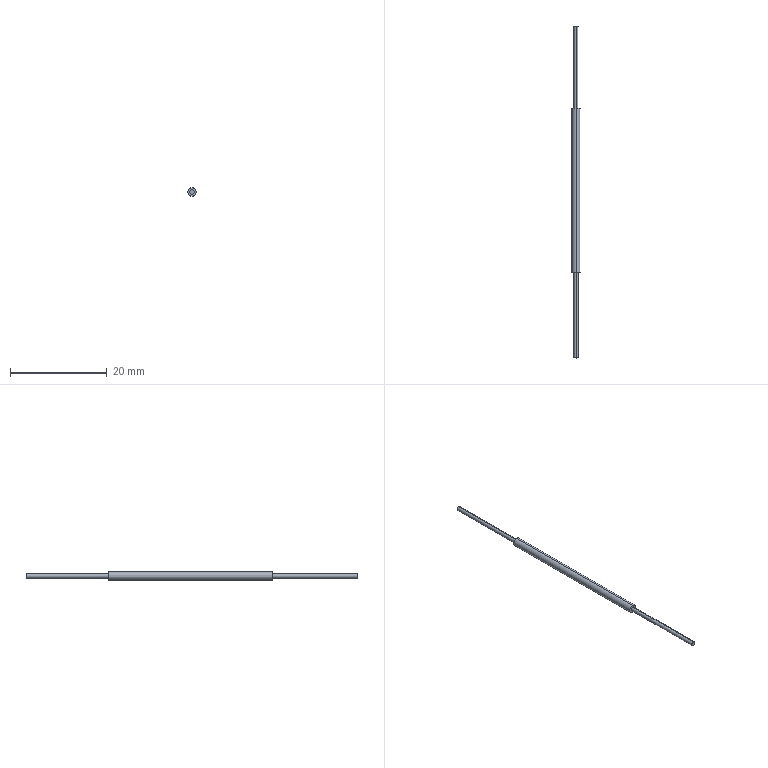Part | SolidWorks | features Revolution 1 | 1 solid | 10 faces | box 1.75 x 68.75 x 1.75 mm | volume 103.887 mm3 | cylinder 6 | plane 4 | commonest cylinder face diameters 0.9 x4 1.75 x2
STEP:
#1=CARTESIAN_POINT('',(0.,67.,-0.45));
#2=VERTEX_POINT('',#1);
#3=CARTESIAN_POINT('',(0.,67.,0.45));
#4=VERTEX_POINT('',#3);
#5=CARTESIAN_POINT('',(0.,67.,0.));
#6=DIRECTION('',(0.,-1.,0.));
#7=DIRECTION('',(0.,0.,-1.));
#8=AXIS2_PLACEMENT_3D('',#5,#6,#7);
#9=CIRCLE('',#8,0.45);
#10=EDGE_CURVE('',#2,#4,#9,.T.);
#11=ORIENTED_EDGE('',*,*,#10,.T.);
#12=CARTESIAN_POINT('',(0.,50.,0.45));
#13=VERTEX_POINT('',#12);
#14=CARTESIAN_POINT('',(0.,-4.379,0.45));
#15=DIRECTION('',(0.,-1.,0.));
#16=VECTOR('',#15,1000.);
#17=LINE('',#14,#16);
#18=EDGE_CURVE('',#4,#13,#17,.T.);
#19=ORIENTED_EDGE('',*,*,#18,.T.);
#20=CARTESIAN_POINT('',(0.,50.,-0.45));
#21=VERTEX_POINT('',#20);
#22=CARTESIAN_POINT('',(0.,50.,0.));
#23=DIRECTION('',(0.,-1.,0.));
#24=DIRECTION('',(0.,0.,-1.));
#25=AXIS2_PLACEMENT_3D('',#22,#23,#24);
#26=CIRCLE('',#25,0.45);
#27=EDGE_CURVE('',#21,#13,#26,.T.);
#28=ORIENTED_EDGE('',*,*,#27,.F.);
#29=CARTESIAN_POINT('',(0.,-4.379,-0.45));
#30=DIRECTION('',(0.,-1.,0.));
#31=VECTOR('',#30,1000.);
#32=LINE('',#29,#31);
#33=EDGE_CURVE('',#2,#21,#32,.T.);
#34=ORIENTED_EDGE('',*,*,#33,.F.);
#35=EDGE_LOOP('',(#11,#19,#28,#34));
#36=FACE_OUTER_BOUND('',#35,.T.);
#37=CARTESIAN_POINT('',(0.,-4.379,0.));
#38=DIRECTION('',(0.,-1.,0.));
#39=DIRECTION('',(0.,0.,-1.));
#40=AXIS2_PLACEMENT_3D('',#37,#38,#39);
#41=CYLINDRICAL_SURFACE('',#40,0.45);
#42=ADVANCED_FACE('',(#36),#41,.T.);
#43=CARTESIAN_POINT('',(0.,50.,-0.875));
#44=VERTEX_POINT('',#43);
#45=CARTESIAN_POINT('',(0.,50.,0.875));
#46=VERTEX_POINT('',#45);
#47=CARTESIAN_POINT('',(0.,50.,0.));
#48=DIRECTION('',(0.,-1.,0.));
#49=DIRECTION('',(0.,0.,-1.));
#50=AXIS2_PLACEMENT_3D('',#47,#48,#49);
#51=CIRCLE('',#50,0.875);
#52=EDGE_CURVE('',#44,#46,#51,.T.);
#53=ORIENTED_EDGE('',*,*,#52,.T.);
#54=CARTESIAN_POINT('',(0.,16.,0.875));
#55=VERTEX_POINT('',#54);
#56=CARTESIAN_POINT('',(0.,-4.379,0.875));
#57=DIRECTION('',(0.,-1.,0.));
#58=VECTOR('',#57,1000.);
#59=LINE('',#56,#58);
#60=EDGE_CURVE('',#46,#55,#59,.T.);
#61=ORIENTED_EDGE('',*,*,#60,.T.);
#62=CARTESIAN_POINT('',(0.,16.,-0.875));
#63=VERTEX_POINT('',#62);
#64=CARTESIAN_POINT('',(0.,16.,0.));
#65=DIRECTION('',(0.,-1.,0.));
#66=DIRECTION('',(0.,0.,-1.));
#67=AXIS2_PLACEMENT_3D('',#64,#65,#66);
#68=CIRCLE('',#67,0.875);
#69=EDGE_CURVE('',#63,#55,#68,.T.);
#70=ORIENTED_EDGE('',*,*,#69,.F.);
#71=CARTESIAN_POINT('',(0.,-4.379,-0.875));
#72=DIRECTION('',(0.,-1.,0.));
#73=VECTOR('',#72,1000.);
#74=LINE('',#71,#73);
#75=EDGE_CURVE('',#44,#63,#74,.T.);
#76=ORIENTED_EDGE('',*,*,#75,.F.);
#77=EDGE_LOOP('',(#53,#61,#70,#76));
#78=FACE_OUTER_BOUND('',#77,.T.);
#79=CARTESIAN_POINT('',(0.,-4.379,0.));
#80=DIRECTION('',(0.,-1.,0.));
#81=DIRECTION('',(0.,0.,-1.));
#82=AXIS2_PLACEMENT_3D('',#79,#80,#81);
#83=CYLINDRICAL_SURFACE('',#82,0.875);
#84=ADVANCED_FACE('',(#78),#83,.T.);
#85=CARTESIAN_POINT('',(0.,16.,-0.45));
#86=VERTEX_POINT('',#85);
#87=CARTESIAN_POINT('',(0.,16.,0.45));
#88=VERTEX_POINT('',#87);
#89=CARTESIAN_POINT('',(0.,16.,0.));
#90=DIRECTION('',(0.,-1.,0.));
#91=DIRECTION('',(0.,0.,-1.));
#92=AXIS2_PLACEMENT_3D('',#89,#90,#91);
#93=CIRCLE('',#92,0.45);
#94=EDGE_CURVE('',#86,#88,#93,.T.);
#95=ORIENTED_EDGE('',*,*,#94,.T.);
#96=CARTESIAN_POINT('',(0.,-1.75,0.45));
#97=VERTEX_POINT('',#96);
#98=CARTESIAN_POINT('',(0.,-4.379,0.45));
#99=DIRECTION('',(0.,-1.,0.));
#100=VECTOR('',#99,1000.);
#101=LINE('',#98,#100);
#102=EDGE_CURVE('',#88,#97,#101,.T.);
#103=ORIENTED_EDGE('',*,*,#102,.T.);
#104=CARTESIAN_POINT('',(0.,-1.75,-0.45));
#105=VERTEX_POINT('',#104);
#106=CARTESIAN_POINT('',(0.,-1.75,0.));
#107=DIRECTION('',(0.,-1.,0.));
#108=DIRECTION('',(0.,0.,-1.));
#109=AXIS2_PLACEMENT_3D('',#106,#107,#108);
#110=CIRCLE('',#109,0.45);
#111=EDGE_CURVE('',#105,#97,#110,.T.);
#112=ORIENTED_EDGE('',*,*,#111,.F.);
#113=CARTESIAN_POINT('',(0.,-4.379,-0.45));
#114=DIRECTION('',(0.,-1.,0.));
#115=VECTOR('',#114,1000.);
#116=LINE('',#113,#115);
#117=EDGE_CURVE('',#86,#105,#116,.T.);
#118=ORIENTED_EDGE('',*,*,#117,.F.);
#119=EDGE_LOOP('',(#95,#103,#112,#118));
#120=FACE_OUTER_BOUND('',#119,.T.);
#121=CARTESIAN_POINT('',(0.,-4.379,0.));
#122=DIRECTION('',(0.,-1.,0.));
#123=DIRECTION('',(0.,0.,-1.));
#124=AXIS2_PLACEMENT_3D('',#121,#122,#123);
#125=CYLINDRICAL_SURFACE('',#124,0.45);
#126=ADVANCED_FACE('',(#120),#125,.T.);
#127=ORIENTED_EDGE('',*,*,#10,.F.);
#128=CARTESIAN_POINT('',(0.,67.,0.));
#129=DIRECTION('',(0.,-1.,0.));
#130=DIRECTION('',(0.,0.,-1.));
#131=AXIS2_PLACEMENT_3D('',#128,#129,#130);
#132=CIRCLE('',#131,0.45);
#133=EDGE_CURVE('',#4,#2,#132,.T.);
#134=ORIENTED_EDGE('',*,*,#133,.F.);
#135=EDGE_LOOP('',(#127,#134));
#136=FACE_OUTER_BOUND('',#135,.T.);
#137=CARTESIAN_POINT('',(0.,67.,-0.45));
#138=DIRECTION('',(0.,1.,0.));
#139=DIRECTION('',(0.,0.,1.));
#140=AXIS2_PLACEMENT_3D('',#137,#138,#139);
#141=PLANE('',#140);
#142=ADVANCED_FACE('',(#136),#141,.T.);
#143=ORIENTED_EDGE('',*,*,#111,.T.);
#144=CARTESIAN_POINT('',(0.,-1.75,0.));
#145=DIRECTION('',(0.,-1.,0.));
#146=DIRECTION('',(0.,0.,-1.));
#147=AXIS2_PLACEMENT_3D('',#144,#145,#146);
#148=CIRCLE('',#147,0.45);
#149=EDGE_CURVE('',#97,#105,#148,.T.);
#150=ORIENTED_EDGE('',*,*,#149,.T.);
#151=EDGE_LOOP('',(#143,#150));
#152=FACE_OUTER_BOUND('',#151,.T.);
#153=CARTESIAN_POINT('',(0.,-1.75,0.));
#154=DIRECTION('',(0.,-1.,0.));
#155=DIRECTION('',(0.,0.,-1.));
#156=AXIS2_PLACEMENT_3D('',#153,#154,#155);
#157=PLANE('',#156);
#158=ADVANCED_FACE('',(#152),#157,.T.);
#159=ORIENTED_EDGE('',*,*,#102,.F.);
#160=CARTESIAN_POINT('',(0.,16.,0.));
#161=DIRECTION('',(0.,-1.,0.));
#162=DIRECTION('',(0.,0.,-1.));
#163=AXIS2_PLACEMENT_3D('',#160,#161,#162);
#164=CIRCLE('',#163,0.45);
#165=EDGE_CURVE('',#88,#86,#164,.T.);
#166=ORIENTED_EDGE('',*,*,#165,.T.);
#167=ORIENTED_EDGE('',*,*,#117,.T.);
#168=ORIENTED_EDGE('',*,*,#149,.F.);
#169=EDGE_LOOP('',(#159,#166,#167,#168));
#170=FACE_OUTER_BOUND('',#169,.T.);
#171=CARTESIAN_POINT('',(0.,-4.379,0.));
#172=DIRECTION('',(0.,-1.,0.));
#173=DIRECTION('',(0.,0.,-1.));
#174=AXIS2_PLACEMENT_3D('',#171,#172,#173);
#175=CYLINDRICAL_SURFACE('',#174,0.45);
#176=ADVANCED_FACE('',(#170),#175,.T.);
#177=ORIENTED_EDGE('',*,*,#69,.T.);
#178=CARTESIAN_POINT('',(0.,16.,0.));
#179=DIRECTION('',(0.,-1.,0.));
#180=DIRECTION('',(0.,0.,-1.));
#181=AXIS2_PLACEMENT_3D('',#178,#179,#180);
#182=CIRCLE('',#181,0.875);
#183=EDGE_CURVE('',#55,#63,#182,.T.);
#184=ORIENTED_EDGE('',*,*,#183,.T.);
#185=EDGE_LOOP('',(#177,#184));
#186=FACE_OUTER_BOUND('',#185,.T.);
#187=ORIENTED_EDGE('',*,*,#94,.F.);
#188=ORIENTED_EDGE('',*,*,#165,.F.);
#189=EDGE_LOOP('',(#187,#188));
#190=FACE_BOUND('',#189,.T.);
#191=CARTESIAN_POINT('',(0.,16.,-0.45));
#192=DIRECTION('',(0.,-1.,0.));
#193=DIRECTION('',(0.,0.,-1.));
#194=AXIS2_PLACEMENT_3D('',#191,#192,#193);
#195=PLANE('',#194);
#196=ADVANCED_FACE('',(#186,#190),#195,.T.);
#197=ORIENTED_EDGE('',*,*,#60,.F.);
#198=CARTESIAN_POINT('',(0.,50.,0.));
#199=DIRECTION('',(0.,-1.,0.));
#200=DIRECTION('',(0.,0.,-1.));
#201=AXIS2_PLACEMENT_3D('',#198,#199,#200);
#202=CIRCLE('',#201,0.875);
#203=EDGE_CURVE('',#46,#44,#202,.T.);
#204=ORIENTED_EDGE('',*,*,#203,.T.);
#205=ORIENTED_EDGE('',*,*,#75,.T.);
#206=ORIENTED_EDGE('',*,*,#183,.F.);
#207=EDGE_LOOP('',(#197,#204,#205,#206));
#208=FACE_OUTER_BOUND('',#207,.T.);
#209=CARTESIAN_POINT('',(0.,-4.379,0.));
#210=DIRECTION('',(0.,-1.,0.));
#211=DIRECTION('',(0.,0.,-1.));
#212=AXIS2_PLACEMENT_3D('',#209,#210,#211);
#213=CYLINDRICAL_SURFACE('',#212,0.875);
#214=ADVANCED_FACE('',(#208),#213,.T.);
#215=ORIENTED_EDGE('',*,*,#27,.T.);
#216=CARTESIAN_POINT('',(0.,50.,0.));
#217=DIRECTION('',(0.,-1.,0.));
#218=DIRECTION('',(0.,0.,-1.));
#219=AXIS2_PLACEMENT_3D('',#216,#217,#218);
#220=CIRCLE('',#219,0.45);
#221=EDGE_CURVE('',#13,#21,#220,.T.);
#222=ORIENTED_EDGE('',*,*,#221,.T.);
#223=EDGE_LOOP('',(#215,#222));
#224=FACE_BOUND('',#223,.T.);
#225=ORIENTED_EDGE('',*,*,#52,.F.);
#226=ORIENTED_EDGE('',*,*,#203,.F.);
#227=EDGE_LOOP('',(#225,#226));
#228=FACE_OUTER_BOUND('',#227,.T.);
#229=CARTESIAN_POINT('',(0.,50.,-0.875));
#230=DIRECTION('',(0.,1.,0.));
#231=DIRECTION('',(0.,0.,1.));
#232=AXIS2_PLACEMENT_3D('',#229,#230,#231);
#233=PLANE('',#232);
#234=ADVANCED_FACE('',(#224,#228),#233,.T.);
#235=ORIENTED_EDGE('',*,*,#18,.F.);
#236=ORIENTED_EDGE('',*,*,#133,.T.);
#237=ORIENTED_EDGE('',*,*,#33,.T.);
#238=ORIENTED_EDGE('',*,*,#221,.F.);
#239=EDGE_LOOP('',(#235,#236,#237,#238));
#240=FACE_OUTER_BOUND('',#239,.T.);
#241=CARTESIAN_POINT('',(0.,-4.379,0.));
#242=DIRECTION('',(0.,-1.,0.));
#243=DIRECTION('',(0.,0.,-1.));
#244=AXIS2_PLACEMENT_3D('',#241,#242,#243);
#245=CYLINDRICAL_SURFACE('',#244,0.45);
#246=ADVANCED_FACE('',(#240),#245,.T.);
#247=CLOSED_SHELL('',(#42,#84,#126,#142,#158,#176,#196,#214,#234,#246));
#248=MANIFOLD_SOLID_BREP('',#247);
#249=CARTESIAN_POINT('',(0.,0.,0.));
#250=DIRECTION('',(0.,0.,1.));
#251=DIRECTION('',(1.,0.,0.));
#252=AXIS2_PLACEMENT_3D('',#249,#250,#251);
#253=(LENGTH_UNIT()NAMED_UNIT(*)SI_UNIT(.MILLI.,.METRE.));
#254=UNCERTAINTY_MEASURE_WITH_UNIT(LENGTH_MEASURE(0.00001),#253,'','');
#255=(NAMED_UNIT(*)PLANE_ANGLE_UNIT()SI_UNIT($,.RADIAN.));
#256=(NAMED_UNIT(*)SI_UNIT($,.STERADIAN.)SOLID_ANGLE_UNIT());
#257=(GEOMETRIC_REPRESENTATION_CONTEXT(3)GLOBAL_UNCERTAINTY_ASSIGNED_CONTEXT((#254))GLOBAL_UNIT_ASSIGNED_CONTEXT((#253,#255,#256))REPRESENTATION_CONTEXT('',''));
#258=ADVANCED_BREP_SHAPE_REPRESENTATION('',(#248,#252),#257);